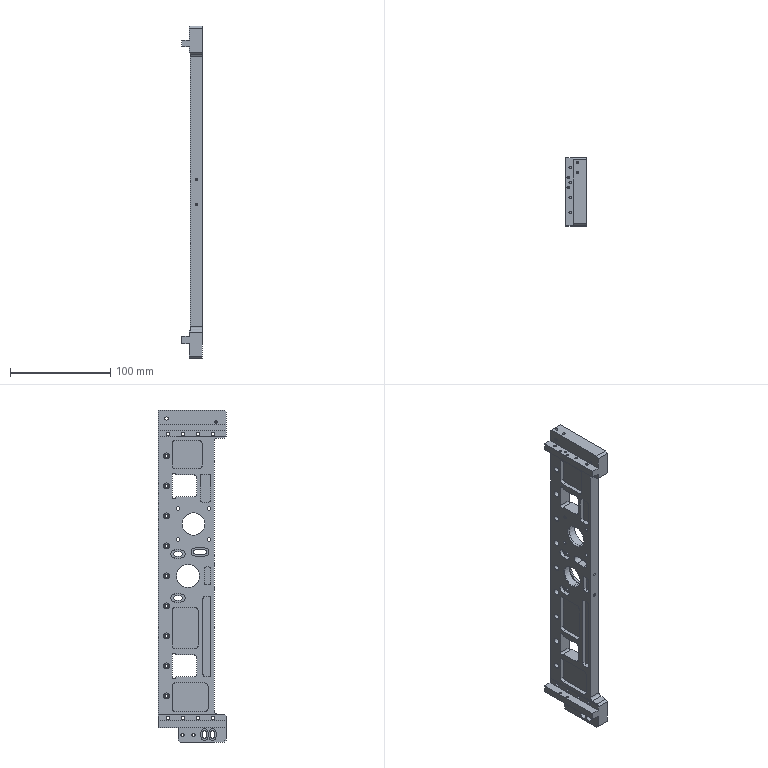Part | NX | features BREP 1 | 1 solid | 413 faces | box 20.5 x 68 x 332 mm | volume 151734 mm3 | cylinder 229 | plane 174 | cone 10 | commonest cylinder face diameters 3.4 x48 6 x48 4 x33 7 x30 2.5 x26 3.3 x8